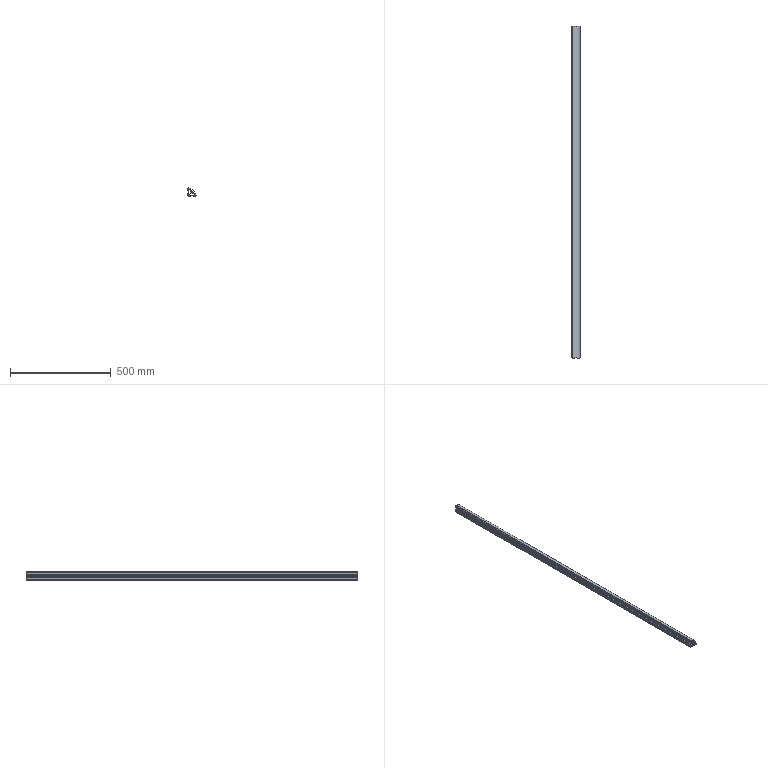Part | 1 solid | 51 faces | box 39.917 x 1650 x 39.917 mm | volume 978005 mm3 | plane 40 | cylinder 11 | commonest cylinder face diameters 4 x3 5 x2 6.8 x2 3 x1 68 x1 76 x1